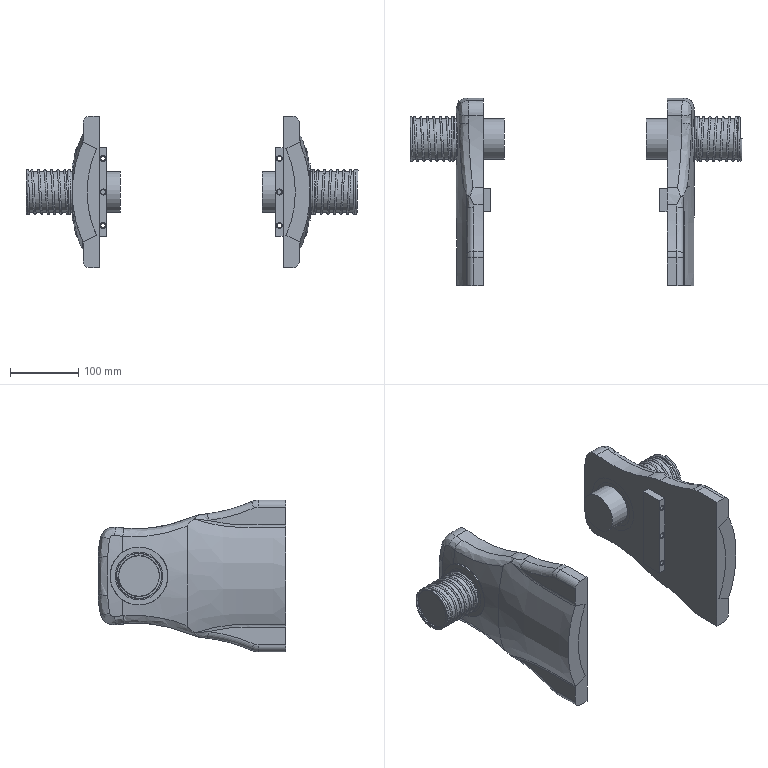Part | NX | features BREP 14 | 14 solids | 178 faces | box 490 x 275.452 x 222.711 mm | volume 3968858 mm3 | cylinder 56 | plane 54 | spline 48 | cone 12 | torus 8 | commonest cylinder face diameters 70 x8 85 x8 7 x6 20 x4 40 x4 48 x4